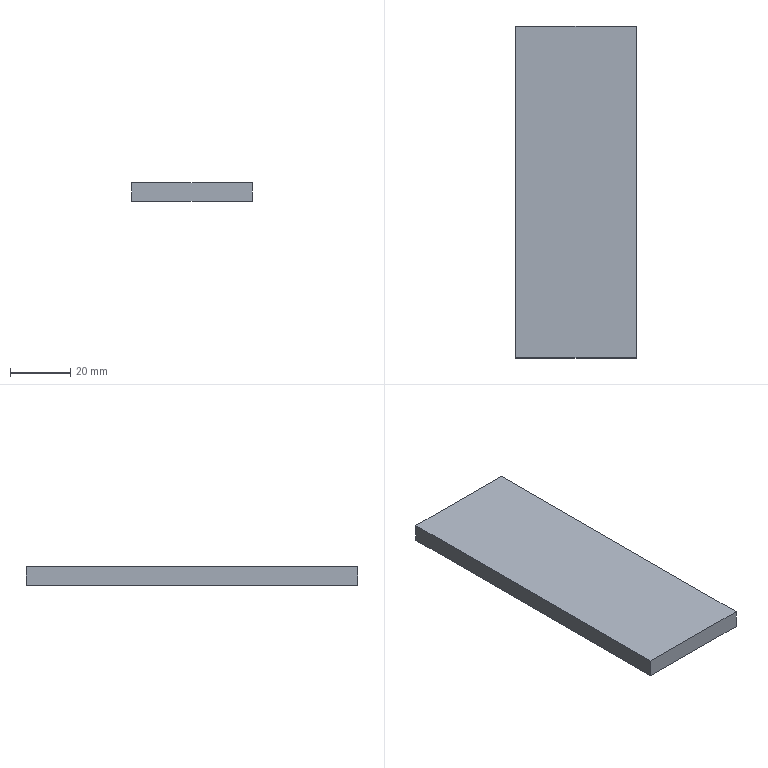Part | SolidWorks | features Extrusion 1 | 1 solid | 6 faces | box 40 x 110 x 6 mm | volume 26400 mm3 | plane 6
STEP:
#1=CARTESIAN_POINT('',(-20.,55.,0.));
#2=VERTEX_POINT('',#1);
#3=CARTESIAN_POINT('',(-20.,-55.,0.));
#4=VERTEX_POINT('',#3);
#5=CARTESIAN_POINT('',(-20.,55.,0.));
#6=DIRECTION('',(0.,-1.,0.));
#7=VECTOR('',#6,1000.);
#8=LINE('',#5,#7);
#9=EDGE_CURVE('',#2,#4,#8,.T.);
#10=ORIENTED_EDGE('',*,*,#9,.T.);
#11=CARTESIAN_POINT('',(-20.,-55.,6.));
#12=VERTEX_POINT('',#11);
#13=CARTESIAN_POINT('',(-20.,-55.,6.));
#14=DIRECTION('',(0.,0.,-1.));
#15=VECTOR('',#14,1000.);
#16=LINE('',#13,#15);
#17=EDGE_CURVE('',#12,#4,#16,.T.);
#18=ORIENTED_EDGE('',*,*,#17,.F.);
#19=CARTESIAN_POINT('',(-20.,55.,6.));
#20=VERTEX_POINT('',#19);
#21=CARTESIAN_POINT('',(-20.,55.,6.));
#22=DIRECTION('',(0.,-1.,0.));
#23=VECTOR('',#22,1000.);
#24=LINE('',#21,#23);
#25=EDGE_CURVE('',#20,#12,#24,.T.);
#26=ORIENTED_EDGE('',*,*,#25,.F.);
#27=CARTESIAN_POINT('',(-20.,55.,6.));
#28=DIRECTION('',(0.,0.,-1.));
#29=VECTOR('',#28,1000.);
#30=LINE('',#27,#29);
#31=EDGE_CURVE('',#20,#2,#30,.T.);
#32=ORIENTED_EDGE('',*,*,#31,.T.);
#33=EDGE_LOOP('',(#10,#18,#26,#32));
#34=FACE_OUTER_BOUND('',#33,.T.);
#35=CARTESIAN_POINT('',(-20.,55.,6.));
#36=DIRECTION('',(1.,0.,0.));
#37=DIRECTION('',(0.,1.,0.));
#38=AXIS2_PLACEMENT_3D('',#35,#36,#37);
#39=PLANE('',#38);
#40=ADVANCED_FACE('',(#34),#39,.F.);
#41=CARTESIAN_POINT('',(20.,-55.,0.));
#42=VERTEX_POINT('',#41);
#43=CARTESIAN_POINT('',(20.,-55.,0.));
#44=DIRECTION('',(1.,0.,0.));
#45=VECTOR('',#44,1000.);
#46=LINE('',#43,#45);
#47=EDGE_CURVE('',#4,#42,#46,.T.);
#48=ORIENTED_EDGE('',*,*,#47,.T.);
#49=CARTESIAN_POINT('',(20.,-55.,6.));
#50=VERTEX_POINT('',#49);
#51=CARTESIAN_POINT('',(20.,-55.,6.));
#52=DIRECTION('',(0.,0.,-1.));
#53=VECTOR('',#52,1000.);
#54=LINE('',#51,#53);
#55=EDGE_CURVE('',#50,#42,#54,.T.);
#56=ORIENTED_EDGE('',*,*,#55,.F.);
#57=CARTESIAN_POINT('',(20.,-55.,6.));
#58=DIRECTION('',(1.,0.,0.));
#59=VECTOR('',#58,1000.);
#60=LINE('',#57,#59);
#61=EDGE_CURVE('',#12,#50,#60,.T.);
#62=ORIENTED_EDGE('',*,*,#61,.F.);
#63=ORIENTED_EDGE('',*,*,#17,.T.);
#64=EDGE_LOOP('',(#48,#56,#62,#63));
#65=FACE_OUTER_BOUND('',#64,.T.);
#66=CARTESIAN_POINT('',(20.,-55.,6.));
#67=DIRECTION('',(0.,1.,0.));
#68=DIRECTION('',(0.,0.,1.));
#69=AXIS2_PLACEMENT_3D('',#66,#67,#68);
#70=PLANE('',#69);
#71=ADVANCED_FACE('',(#65),#70,.F.);
#72=CARTESIAN_POINT('',(20.,55.,0.));
#73=VERTEX_POINT('',#72);
#74=CARTESIAN_POINT('',(20.,55.,0.));
#75=DIRECTION('',(0.,1.,0.));
#76=VECTOR('',#75,1000.);
#77=LINE('',#74,#76);
#78=EDGE_CURVE('',#42,#73,#77,.T.);
#79=ORIENTED_EDGE('',*,*,#78,.T.);
#80=CARTESIAN_POINT('',(20.,55.,6.));
#81=VERTEX_POINT('',#80);
#82=CARTESIAN_POINT('',(20.,55.,6.));
#83=DIRECTION('',(0.,0.,-1.));
#84=VECTOR('',#83,1000.);
#85=LINE('',#82,#84);
#86=EDGE_CURVE('',#81,#73,#85,.T.);
#87=ORIENTED_EDGE('',*,*,#86,.F.);
#88=CARTESIAN_POINT('',(20.,55.,6.));
#89=DIRECTION('',(0.,1.,0.));
#90=VECTOR('',#89,1000.);
#91=LINE('',#88,#90);
#92=EDGE_CURVE('',#50,#81,#91,.T.);
#93=ORIENTED_EDGE('',*,*,#92,.F.);
#94=ORIENTED_EDGE('',*,*,#55,.T.);
#95=EDGE_LOOP('',(#79,#87,#93,#94));
#96=FACE_OUTER_BOUND('',#95,.T.);
#97=CARTESIAN_POINT('',(20.,55.,6.));
#98=DIRECTION('',(-1.,0.,0.));
#99=DIRECTION('',(0.,-1.,0.));
#100=AXIS2_PLACEMENT_3D('',#97,#98,#99);
#101=PLANE('',#100);
#102=ADVANCED_FACE('',(#96),#101,.F.);
#103=CARTESIAN_POINT('',(20.,55.,0.));
#104=DIRECTION('',(-1.,0.,0.));
#105=VECTOR('',#104,1000.);
#106=LINE('',#103,#105);
#107=EDGE_CURVE('',#73,#2,#106,.T.);
#108=ORIENTED_EDGE('',*,*,#107,.T.);
#109=ORIENTED_EDGE('',*,*,#31,.F.);
#110=CARTESIAN_POINT('',(20.,55.,6.));
#111=DIRECTION('',(-1.,0.,0.));
#112=VECTOR('',#111,1000.);
#113=LINE('',#110,#112);
#114=EDGE_CURVE('',#81,#20,#113,.T.);
#115=ORIENTED_EDGE('',*,*,#114,.F.);
#116=ORIENTED_EDGE('',*,*,#86,.T.);
#117=EDGE_LOOP('',(#108,#109,#115,#116));
#118=FACE_OUTER_BOUND('',#117,.T.);
#119=CARTESIAN_POINT('',(20.,55.,6.));
#120=DIRECTION('',(0.,-1.,0.));
#121=DIRECTION('',(0.,0.,-1.));
#122=AXIS2_PLACEMENT_3D('',#119,#120,#121);
#123=PLANE('',#122);
#124=ADVANCED_FACE('',(#118),#123,.F.);
#125=ORIENTED_EDGE('',*,*,#25,.T.);
#126=ORIENTED_EDGE('',*,*,#61,.T.);
#127=ORIENTED_EDGE('',*,*,#92,.T.);
#128=ORIENTED_EDGE('',*,*,#114,.T.);
#129=EDGE_LOOP('',(#125,#126,#127,#128));
#130=FACE_OUTER_BOUND('',#129,.T.);
#131=CARTESIAN_POINT('',(0.,0.,6.));
#132=DIRECTION('',(0.,0.,-1.));
#133=DIRECTION('',(-1.,0.,0.));
#134=AXIS2_PLACEMENT_3D('',#131,#132,#133);
#135=PLANE('',#134);
#136=ADVANCED_FACE('',(#130),#135,.F.);
#137=ORIENTED_EDGE('',*,*,#9,.F.);
#138=ORIENTED_EDGE('',*,*,#107,.F.);
#139=ORIENTED_EDGE('',*,*,#78,.F.);
#140=ORIENTED_EDGE('',*,*,#47,.F.);
#141=EDGE_LOOP('',(#137,#138,#139,#140));
#142=FACE_OUTER_BOUND('',#141,.T.);
#143=CARTESIAN_POINT('',(0.,0.,0.));
#144=DIRECTION('',(0.,0.,-1.));
#145=DIRECTION('',(-1.,0.,0.));
#146=AXIS2_PLACEMENT_3D('',#143,#144,#145);
#147=PLANE('',#146);
#148=ADVANCED_FACE('',(#142),#147,.T.);
#149=CLOSED_SHELL('',(#40,#71,#102,#124,#136,#148));
#150=MANIFOLD_SOLID_BREP('',#149);
#151=CARTESIAN_POINT('',(0.,0.,0.));
#152=DIRECTION('',(0.,0.,1.));
#153=DIRECTION('',(1.,0.,0.));
#154=AXIS2_PLACEMENT_3D('',#151,#152,#153);
#155=(LENGTH_UNIT()NAMED_UNIT(*)SI_UNIT(.MILLI.,.METRE.));
#156=UNCERTAINTY_MEASURE_WITH_UNIT(LENGTH_MEASURE(0.00001),#155,'','');
#157=(NAMED_UNIT(*)PLANE_ANGLE_UNIT()SI_UNIT($,.RADIAN.));
#158=(NAMED_UNIT(*)SI_UNIT($,.STERADIAN.)SOLID_ANGLE_UNIT());
#159=(GEOMETRIC_REPRESENTATION_CONTEXT(3)GLOBAL_UNCERTAINTY_ASSIGNED_CONTEXT((#156))GLOBAL_UNIT_ASSIGNED_CONTEXT((#155,#157,#158))REPRESENTATION_CONTEXT('',''));
#160=ADVANCED_BREP_SHAPE_REPRESENTATION('',(#150,#154),#159);